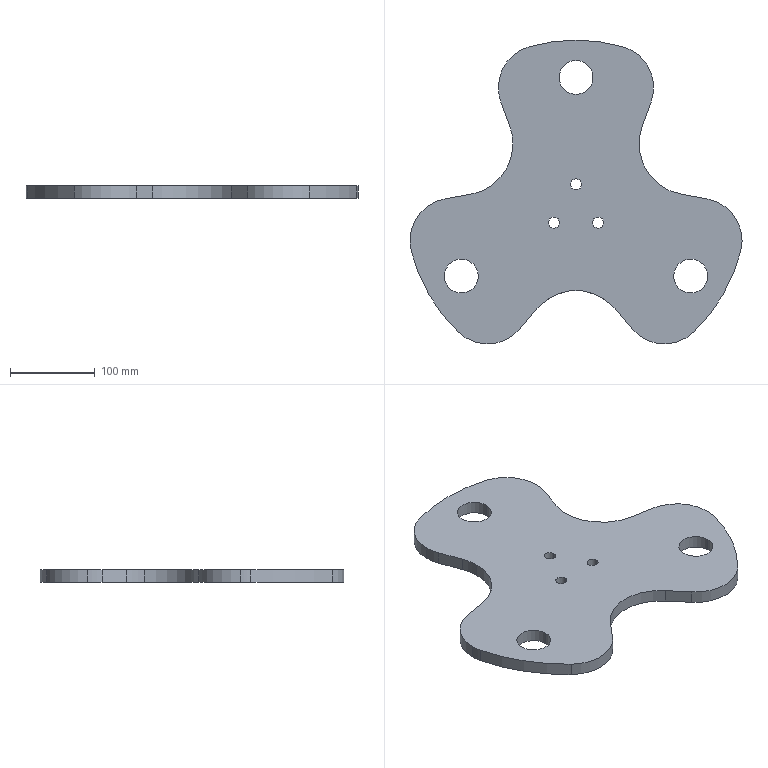Part | SolidWorks | features ICE 2, Extrusion 1, Fillet 1 | 1 solid | 35 faces | box 391.135 x 357.967 x 15 mm | volume 1196806 mm3 | cylinder 27 | plane 8 | commonest cylinder face diameters 100 x8 13 x6 40 x6 120 x4 400 x3
STEP:
#1=CARTESIAN_POINT('',(-6.5,30.,0.));
#2=VERTEX_POINT('',#1);
#3=CARTESIAN_POINT('',(6.5,30.,0.));
#4=VERTEX_POINT('',#3);
#5=CARTESIAN_POINT('',(0.,30.,0.));
#6=DIRECTION('',(0.,0.,1.));
#7=DIRECTION('',(1.,0.,0.));
#8=AXIS2_PLACEMENT_3D('',#5,#6,#7);
#9=CIRCLE('',#8,6.5);
#10=EDGE_CURVE('',#2,#4,#9,.T.);
#11=ORIENTED_EDGE('',*,*,#10,.F.);
#12=CARTESIAN_POINT('',(-6.5,30.,15.));
#13=VERTEX_POINT('',#12);
#14=CARTESIAN_POINT('',(-6.5,30.,-35.));
#15=DIRECTION('',(0.,0.,1.));
#16=VECTOR('',#15,1000.);
#17=LINE('',#14,#16);
#18=EDGE_CURVE('',#2,#13,#17,.T.);
#19=ORIENTED_EDGE('',*,*,#18,.T.);
#20=CARTESIAN_POINT('',(6.5,30.,15.));
#21=VERTEX_POINT('',#20);
#22=CARTESIAN_POINT('',(0.,30.,15.));
#23=DIRECTION('',(0.,0.,1.));
#24=DIRECTION('',(1.,0.,0.));
#25=AXIS2_PLACEMENT_3D('',#22,#23,#24);
#26=CIRCLE('',#25,6.5);
#27=EDGE_CURVE('',#13,#21,#26,.T.);
#28=ORIENTED_EDGE('',*,*,#27,.T.);
#29=CARTESIAN_POINT('',(6.5,30.,-35.));
#30=DIRECTION('',(0.,0.,1.));
#31=VECTOR('',#30,1000.);
#32=LINE('',#29,#31);
#33=EDGE_CURVE('',#4,#21,#32,.T.);
#34=ORIENTED_EDGE('',*,*,#33,.F.);
#35=EDGE_LOOP('',(#11,#19,#28,#34));
#36=FACE_OUTER_BOUND('',#35,.T.);
#37=CARTESIAN_POINT('',(0.,30.,-35.));
#38=DIRECTION('',(0.,0.,1.));
#39=DIRECTION('',(1.,0.,0.));
#40=AXIS2_PLACEMENT_3D('',#37,#38,#39);
#41=CYLINDRICAL_SURFACE('',#40,6.5);
#42=ADVANCED_FACE('',(#36),#41,.F.);
#43=CARTESIAN_POINT('',(19.481,-15.,0.));
#44=VERTEX_POINT('',#43);
#45=CARTESIAN_POINT('',(32.481,-15.,0.));
#46=VERTEX_POINT('',#45);
#47=CARTESIAN_POINT('',(25.981,-15.,0.));
#48=DIRECTION('',(0.,0.,1.));
#49=DIRECTION('',(1.,0.,0.));
#50=AXIS2_PLACEMENT_3D('',#47,#48,#49);
#51=CIRCLE('',#50,6.5);
#52=EDGE_CURVE('',#44,#46,#51,.T.);
#53=ORIENTED_EDGE('',*,*,#52,.F.);
#54=CARTESIAN_POINT('',(19.481,-15.,15.));
#55=VERTEX_POINT('',#54);
#56=CARTESIAN_POINT('',(19.481,-15.,-35.));
#57=DIRECTION('',(0.,0.,1.));
#58=VECTOR('',#57,1000.);
#59=LINE('',#56,#58);
#60=EDGE_CURVE('',#44,#55,#59,.T.);
#61=ORIENTED_EDGE('',*,*,#60,.T.);
#62=CARTESIAN_POINT('',(32.481,-15.,15.));
#63=VERTEX_POINT('',#62);
#64=CARTESIAN_POINT('',(25.981,-15.,15.));
#65=DIRECTION('',(0.,0.,1.));
#66=DIRECTION('',(1.,0.,0.));
#67=AXIS2_PLACEMENT_3D('',#64,#65,#66);
#68=CIRCLE('',#67,6.5);
#69=EDGE_CURVE('',#55,#63,#68,.T.);
#70=ORIENTED_EDGE('',*,*,#69,.T.);
#71=CARTESIAN_POINT('',(32.481,-15.,-35.));
#72=DIRECTION('',(0.,0.,1.));
#73=VECTOR('',#72,1000.);
#74=LINE('',#71,#73);
#75=EDGE_CURVE('',#46,#63,#74,.T.);
#76=ORIENTED_EDGE('',*,*,#75,.F.);
#77=EDGE_LOOP('',(#53,#61,#70,#76));
#78=FACE_OUTER_BOUND('',#77,.T.);
#79=CARTESIAN_POINT('',(25.981,-15.,-35.));
#80=DIRECTION('',(0.,0.,1.));
#81=DIRECTION('',(1.,0.,0.));
#82=AXIS2_PLACEMENT_3D('',#79,#80,#81);
#83=CYLINDRICAL_SURFACE('',#82,6.5);
#84=ADVANCED_FACE('',(#78),#83,.F.);
#85=CARTESIAN_POINT('',(-32.481,-15.,0.));
#86=VERTEX_POINT('',#85);
#87=CARTESIAN_POINT('',(-19.481,-15.,0.));
#88=VERTEX_POINT('',#87);
#89=CARTESIAN_POINT('',(-25.981,-15.,0.));
#90=DIRECTION('',(0.,0.,1.));
#91=DIRECTION('',(1.,0.,0.));
#92=AXIS2_PLACEMENT_3D('',#89,#90,#91);
#93=CIRCLE('',#92,6.5);
#94=EDGE_CURVE('',#86,#88,#93,.T.);
#95=ORIENTED_EDGE('',*,*,#94,.F.);
#96=CARTESIAN_POINT('',(-32.481,-15.,15.));
#97=VERTEX_POINT('',#96);
#98=CARTESIAN_POINT('',(-32.481,-15.,-35.));
#99=DIRECTION('',(0.,0.,1.));
#100=VECTOR('',#99,1000.);
#101=LINE('',#98,#100);
#102=EDGE_CURVE('',#86,#97,#101,.T.);
#103=ORIENTED_EDGE('',*,*,#102,.T.);
#104=CARTESIAN_POINT('',(-19.481,-15.,15.));
#105=VERTEX_POINT('',#104);
#106=CARTESIAN_POINT('',(-25.981,-15.,15.));
#107=DIRECTION('',(0.,0.,1.));
#108=DIRECTION('',(1.,0.,0.));
#109=AXIS2_PLACEMENT_3D('',#106,#107,#108);
#110=CIRCLE('',#109,6.5);
#111=EDGE_CURVE('',#97,#105,#110,.T.);
#112=ORIENTED_EDGE('',*,*,#111,.T.);
#113=CARTESIAN_POINT('',(-19.481,-15.,-35.));
#114=DIRECTION('',(0.,0.,1.));
#115=VECTOR('',#114,1000.);
#116=LINE('',#113,#115);
#117=EDGE_CURVE('',#88,#105,#116,.T.);
#118=ORIENTED_EDGE('',*,*,#117,.F.);
#119=EDGE_LOOP('',(#95,#103,#112,#118));
#120=FACE_OUTER_BOUND('',#119,.T.);
#121=CARTESIAN_POINT('',(-25.981,-15.,-35.));
#122=DIRECTION('',(0.,0.,1.));
#123=DIRECTION('',(1.,0.,0.));
#124=AXIS2_PLACEMENT_3D('',#121,#122,#123);
#125=CYLINDRICAL_SURFACE('',#124,6.5);
#126=ADVANCED_FACE('',(#120),#125,.F.);
#127=CARTESIAN_POINT('',(-91.438,144.163,15.));
#128=VERTEX_POINT('',#127);
#129=CARTESIAN_POINT('',(-88.422,127.062,15.));
#130=VERTEX_POINT('',#129);
#131=CARTESIAN_POINT('',(-41.438,144.163,15.));
#132=DIRECTION('',(0.,0.,1.));
#133=DIRECTION('',(1.,0.,0.));
#134=AXIS2_PLACEMENT_3D('',#131,#132,#133);
#135=CIRCLE('',#134,50.);
#136=EDGE_CURVE('',#128,#130,#135,.T.);
#137=ORIENTED_EDGE('',*,*,#136,.F.);
#138=CARTESIAN_POINT('',(-91.438,144.163,0.));
#139=VERTEX_POINT('',#138);
#140=CARTESIAN_POINT('',(-91.438,144.163,15.));
#141=DIRECTION('',(0.,0.,-1.));
#142=VECTOR('',#141,1000.);
#143=LINE('',#140,#142);
#144=EDGE_CURVE('',#128,#139,#143,.T.);
#145=ORIENTED_EDGE('',*,*,#144,.T.);
#146=CARTESIAN_POINT('',(-88.422,127.062,0.));
#147=VERTEX_POINT('',#146);
#148=CARTESIAN_POINT('',(-41.438,144.163,0.));
#149=DIRECTION('',(0.,0.,-1.));
#150=DIRECTION('',(1.,0.,0.));
#151=AXIS2_PLACEMENT_3D('',#148,#149,#150);
#152=CIRCLE('',#151,50.);
#153=EDGE_CURVE('',#147,#139,#152,.T.);
#154=ORIENTED_EDGE('',*,*,#153,.F.);
#155=CARTESIAN_POINT('',(-88.422,127.062,-15.));
#156=DIRECTION('',(0.,0.,-1.));
#157=VECTOR('',#156,1000.);
#158=LINE('',#155,#157);
#159=EDGE_CURVE('',#130,#147,#158,.T.);
#160=ORIENTED_EDGE('',*,*,#159,.F.);
#161=EDGE_LOOP('',(#137,#145,#154,#160));
#162=FACE_OUTER_BOUND('',#161,.T.);
#163=CARTESIAN_POINT('',(-41.438,144.163,15.));
#164=DIRECTION('',(0.,0.,-1.));
#165=DIRECTION('',(-1.,0.,0.));
#166=AXIS2_PLACEMENT_3D('',#163,#164,#165);
#167=CYLINDRICAL_SURFACE('',#166,50.);
#168=ADVANCED_FACE('',(#162),#167,.T.);
#169=CARTESIAN_POINT('',(-195.568,-36.195,15.));
#170=VERTEX_POINT('',#169);
#171=CARTESIAN_POINT('',(-194.09,-48.26,15.));
#172=VERTEX_POINT('',#171);
#173=CARTESIAN_POINT('',(-145.568,-36.195,15.));
#174=DIRECTION('',(0.,0.,1.));
#175=DIRECTION('',(1.,0.,0.));
#176=AXIS2_PLACEMENT_3D('',#173,#174,#175);
#177=CIRCLE('',#176,50.);
#178=EDGE_CURVE('',#170,#172,#177,.T.);
#179=ORIENTED_EDGE('',*,*,#178,.F.);
#180=CARTESIAN_POINT('',(-195.568,-36.195,0.));
#181=VERTEX_POINT('',#180);
#182=CARTESIAN_POINT('',(-195.568,-36.195,15.));
#183=DIRECTION('',(0.,0.,-1.));
#184=VECTOR('',#183,1000.);
#185=LINE('',#182,#184);
#186=EDGE_CURVE('',#170,#181,#185,.T.);
#187=ORIENTED_EDGE('',*,*,#186,.T.);
#188=CARTESIAN_POINT('',(-194.09,-48.26,0.));
#189=VERTEX_POINT('',#188);
#190=CARTESIAN_POINT('',(-145.568,-36.195,0.));
#191=DIRECTION('',(0.,0.,-1.));
#192=DIRECTION('',(1.,0.,0.));
#193=AXIS2_PLACEMENT_3D('',#190,#191,#192);
#194=CIRCLE('',#193,50.);
#195=EDGE_CURVE('',#189,#181,#194,.T.);
#196=ORIENTED_EDGE('',*,*,#195,.F.);
#197=CARTESIAN_POINT('',(-194.09,-48.26,15.));
#198=DIRECTION('',(0.,0.,-1.));
#199=VECTOR('',#198,1000.);
#200=LINE('',#197,#199);
#201=EDGE_CURVE('',#172,#189,#200,.T.);
#202=ORIENTED_EDGE('',*,*,#201,.F.);
#203=EDGE_LOOP('',(#179,#187,#196,#202));
#204=FACE_OUTER_BOUND('',#203,.T.);
#205=CARTESIAN_POINT('',(-145.568,-36.195,15.));
#206=DIRECTION('',(0.,0.,-1.));
#207=DIRECTION('',(-1.,0.,0.));
#208=AXIS2_PLACEMENT_3D('',#205,#206,#207);
#209=CYLINDRICAL_SURFACE('',#208,50.);
#210=ADVANCED_FACE('',(#204),#209,.T.);
#211=CARTESIAN_POINT('',(-74.234,77.5,0.));
#212=VERTEX_POINT('',#211);
#213=CARTESIAN_POINT('',(-77.852,98.021,0.));
#214=VERTEX_POINT('',#213);
#215=CARTESIAN_POINT('',(-134.234,77.5,0.));
#216=DIRECTION('',(0.,0.,1.));
#217=DIRECTION('',(1.,0.,0.));
#218=AXIS2_PLACEMENT_3D('',#215,#216,#217);
#219=CIRCLE('',#218,60.);
#220=EDGE_CURVE('',#212,#214,#219,.T.);
#221=ORIENTED_EDGE('',*,*,#220,.F.);
#222=CARTESIAN_POINT('',(-74.234,77.5,15.));
#223=VERTEX_POINT('',#222);
#224=CARTESIAN_POINT('',(-74.234,77.5,-15.));
#225=DIRECTION('',(0.,0.,1.));
#226=VECTOR('',#225,1000.);
#227=LINE('',#224,#226);
#228=EDGE_CURVE('',#212,#223,#227,.T.);
#229=ORIENTED_EDGE('',*,*,#228,.T.);
#230=CARTESIAN_POINT('',(-77.852,98.021,15.));
#231=VERTEX_POINT('',#230);
#232=CARTESIAN_POINT('',(-134.234,77.5,15.));
#233=DIRECTION('',(0.,0.,1.));
#234=DIRECTION('',(-1.,0.,0.));
#235=AXIS2_PLACEMENT_3D('',#232,#233,#234);
#236=CIRCLE('',#235,60.);
#237=EDGE_CURVE('',#223,#231,#236,.T.);
#238=ORIENTED_EDGE('',*,*,#237,.T.);
#239=CARTESIAN_POINT('',(-77.852,98.021,-15.));
#240=DIRECTION('',(0.,0.,1.));
#241=VECTOR('',#240,1000.);
#242=LINE('',#239,#241);
#243=EDGE_CURVE('',#214,#231,#242,.T.);
#244=ORIENTED_EDGE('',*,*,#243,.F.);
#245=EDGE_LOOP('',(#221,#229,#238,#244));
#246=FACE_OUTER_BOUND('',#245,.T.);
#247=CARTESIAN_POINT('',(-134.234,77.5,-15.));
#248=DIRECTION('',(0.,0.,1.));
#249=DIRECTION('',(1.,0.,0.));
#250=AXIS2_PLACEMENT_3D('',#247,#248,#249);
#251=CYLINDRICAL_SURFACE('',#250,60.);
#252=ADVANCED_FACE('',(#246),#251,.F.);
#253=CARTESIAN_POINT('',(-155.1,-78.,15.));
#254=VERTEX_POINT('',#253);
#255=CARTESIAN_POINT('',(-115.1,-78.,15.));
#256=VERTEX_POINT('',#255);
#257=CARTESIAN_POINT('',(-135.1,-78.,15.));
#258=DIRECTION('',(0.,0.,1.));
#259=DIRECTION('',(1.,0.,0.));
#260=AXIS2_PLACEMENT_3D('',#257,#258,#259);
#261=CIRCLE('',#260,20.);
#262=EDGE_CURVE('',#254,#256,#261,.T.);
#263=ORIENTED_EDGE('',*,*,#262,.T.);
#264=CARTESIAN_POINT('',(-115.1,-78.,0.));
#265=VERTEX_POINT('',#264);
#266=CARTESIAN_POINT('',(-115.1,-78.,15.));
#267=DIRECTION('',(0.,0.,-1.));
#268=VECTOR('',#267,1000.);
#269=LINE('',#266,#268);
#270=EDGE_CURVE('',#256,#265,#269,.T.);
#271=ORIENTED_EDGE('',*,*,#270,.T.);
#272=CARTESIAN_POINT('',(-155.1,-78.,0.));
#273=VERTEX_POINT('',#272);
#274=CARTESIAN_POINT('',(-135.1,-78.,0.));
#275=DIRECTION('',(0.,0.,1.));
#276=DIRECTION('',(1.,0.,0.));
#277=AXIS2_PLACEMENT_3D('',#274,#275,#276);
#278=CIRCLE('',#277,20.);
#279=EDGE_CURVE('',#273,#265,#278,.T.);
#280=ORIENTED_EDGE('',*,*,#279,.F.);
#281=CARTESIAN_POINT('',(-155.1,-78.,15.));
#282=DIRECTION('',(0.,0.,-1.));
#283=VECTOR('',#282,1000.);
#284=LINE('',#281,#283);
#285=EDGE_CURVE('',#254,#273,#284,.T.);
#286=ORIENTED_EDGE('',*,*,#285,.F.);
#287=EDGE_LOOP('',(#263,#271,#280,#286));
#288=FACE_OUTER_BOUND('',#287,.T.);
#289=CARTESIAN_POINT('',(-135.1,-78.,15.));
#290=DIRECTION('',(0.,0.,-1.));
#291=DIRECTION('',(-1.,0.,0.));
#292=AXIS2_PLACEMENT_3D('',#289,#290,#291);
#293=CYLINDRICAL_SURFACE('',#292,20.);
#294=ADVANCED_FACE('',(#288),#293,.F.);
#295=CARTESIAN_POINT('',(115.1,-78.,15.));
#296=VERTEX_POINT('',#295);
#297=CARTESIAN_POINT('',(155.1,-78.,15.));
#298=VERTEX_POINT('',#297);
#299=CARTESIAN_POINT('',(135.1,-78.,15.));
#300=DIRECTION('',(0.,0.,1.));
#301=DIRECTION('',(1.,0.,0.));
#302=AXIS2_PLACEMENT_3D('',#299,#300,#301);
#303=CIRCLE('',#302,20.);
#304=EDGE_CURVE('',#296,#298,#303,.T.);
#305=ORIENTED_EDGE('',*,*,#304,.T.);
#306=CARTESIAN_POINT('',(155.1,-78.,0.));
#307=VERTEX_POINT('',#306);
#308=CARTESIAN_POINT('',(155.1,-78.,15.));
#309=DIRECTION('',(0.,0.,-1.));
#310=VECTOR('',#309,1000.);
#311=LINE('',#308,#310);
#312=EDGE_CURVE('',#298,#307,#311,.T.);
#313=ORIENTED_EDGE('',*,*,#312,.T.);
#314=CARTESIAN_POINT('',(115.1,-78.,0.));
#315=VERTEX_POINT('',#314);
#316=CARTESIAN_POINT('',(135.1,-78.,0.));
#317=DIRECTION('',(0.,0.,1.));
#318=DIRECTION('',(1.,0.,0.));
#319=AXIS2_PLACEMENT_3D('',#316,#317,#318);
#320=CIRCLE('',#319,20.);
#321=EDGE_CURVE('',#315,#307,#320,.T.);
#322=ORIENTED_EDGE('',*,*,#321,.F.);
#323=CARTESIAN_POINT('',(115.1,-78.,15.));
#324=DIRECTION('',(0.,0.,-1.));
#325=VECTOR('',#324,1000.);
#326=LINE('',#323,#325);
#327=EDGE_CURVE('',#296,#315,#326,.T.);
#328=ORIENTED_EDGE('',*,*,#327,.F.);
#329=EDGE_LOOP('',(#305,#313,#322,#328));
#330=FACE_OUTER_BOUND('',#329,.T.);
#331=CARTESIAN_POINT('',(135.1,-78.,15.));
#332=DIRECTION('',(0.,0.,-1.));
#333=DIRECTION('',(-1.,0.,0.));
#334=AXIS2_PLACEMENT_3D('',#331,#332,#333);
#335=CYLINDRICAL_SURFACE('',#334,20.);
#336=ADVANCED_FACE('',(#330),#335,.F.);
#337=CARTESIAN_POINT('',(-20.,156.,15.));
#338=VERTEX_POINT('',#337);
#339=CARTESIAN_POINT('',(20.,156.,15.));
#340=VERTEX_POINT('',#339);
#341=CARTESIAN_POINT('',(0.,156.,15.));
#342=DIRECTION('',(0.,0.,1.));
#343=DIRECTION('',(1.,0.,0.));
#344=AXIS2_PLACEMENT_3D('',#341,#342,#343);
#345=CIRCLE('',#344,20.);
#346=EDGE_CURVE('',#338,#340,#345,.T.);
#347=ORIENTED_EDGE('',*,*,#346,.T.);
#348=CARTESIAN_POINT('',(20.,156.,0.));
#349=VERTEX_POINT('',#348);
#350=CARTESIAN_POINT('',(20.,156.,15.));
#351=DIRECTION('',(0.,0.,-1.));
#352=VECTOR('',#351,1000.);
#353=LINE('',#350,#352);
#354=EDGE_CURVE('',#340,#349,#353,.T.);
#355=ORIENTED_EDGE('',*,*,#354,.T.);
#356=CARTESIAN_POINT('',(-20.,156.,0.));
#357=VERTEX_POINT('',#356);
#358=CARTESIAN_POINT('',(0.,156.,0.));
#359=DIRECTION('',(0.,0.,1.));
#360=DIRECTION('',(1.,0.,0.));
#361=AXIS2_PLACEMENT_3D('',#358,#359,#360);
#362=CIRCLE('',#361,20.);
#363=EDGE_CURVE('',#357,#349,#362,.T.);
#364=ORIENTED_EDGE('',*,*,#363,.F.);
#365=CARTESIAN_POINT('',(-20.,156.,15.));
#366=DIRECTION('',(0.,0.,-1.));
#367=VECTOR('',#366,1000.);
#368=LINE('',#365,#367);
#369=EDGE_CURVE('',#338,#357,#368,.T.);
#370=ORIENTED_EDGE('',*,*,#369,.F.);
#371=EDGE_LOOP('',(#347,#355,#364,#370));
#372=FACE_OUTER_BOUND('',#371,.T.);
#373=CARTESIAN_POINT('',(0.,156.,15.));
#374=DIRECTION('',(0.,0.,-1.));
#375=DIRECTION('',(-1.,0.,0.));
#376=AXIS2_PLACEMENT_3D('',#373,#374,#375);
#377=CYLINDRICAL_SURFACE('',#376,20.);
#378=ADVANCED_FACE('',(#372),#377,.F.);
#379=CARTESIAN_POINT('',(138.84,-143.957,15.));
#380=VERTEX_POINT('',#379);
#381=CARTESIAN_POINT('',(194.09,-48.26,15.));
#382=VERTEX_POINT('',#381);
#383=CARTESIAN_POINT('',(0.,0.,15.));
#384=DIRECTION('',(0.,0.,1.));
#385=DIRECTION('',(1.,0.,0.));
#386=AXIS2_PLACEMENT_3D('',#383,#384,#385);
#387=CIRCLE('',#386,200.);
#388=EDGE_CURVE('',#380,#382,#387,.T.);
#389=ORIENTED_EDGE('',*,*,#388,.F.);
#390=CARTESIAN_POINT('',(138.84,-143.957,0.));
#391=VERTEX_POINT('',#390);
#392=CARTESIAN_POINT('',(138.84,-143.957,15.));
#393=DIRECTION('',(0.,0.,-1.));
#394=VECTOR('',#393,1000.);
#395=LINE('',#392,#394);
#396=EDGE_CURVE('',#380,#391,#395,.T.);
#397=ORIENTED_EDGE('',*,*,#396,.T.);
#398=CARTESIAN_POINT('',(194.09,-48.26,0.));
#399=VERTEX_POINT('',#398);
#400=CARTESIAN_POINT('',(0.,0.,0.));
#401=DIRECTION('',(0.,0.,1.));
#402=DIRECTION('',(1.,0.,0.));
#403=AXIS2_PLACEMENT_3D('',#400,#401,#402);
#404=CIRCLE('',#403,200.);
#405=EDGE_CURVE('',#391,#399,#404,.T.);
#406=ORIENTED_EDGE('',*,*,#405,.T.);
#407=CARTESIAN_POINT('',(194.09,-48.26,15.));
#408=DIRECTION('',(0.,0.,1.));
#409=VECTOR('',#408,1000.);
#410=LINE('',#407,#409);
#411=EDGE_CURVE('',#399,#382,#410,.T.);
#412=ORIENTED_EDGE('',*,*,#411,.T.);
#413=EDGE_LOOP('',(#389,#397,#406,#412));
#414=FACE_OUTER_BOUND('',#413,.T.);
#415=CARTESIAN_POINT('',(0.,0.,15.));
#416=DIRECTION('',(0.,0.,-1.));
#417=DIRECTION('',(-1.,0.,0.));
#418=AXIS2_PLACEMENT_3D('',#415,#416,#417);
#419=CYLINDRICAL_SURFACE('',#418,200.);
#420=ADVANCED_FACE('',(#414),#419,.T.);
#421=CARTESIAN_POINT('',(-138.84,-143.957,0.));
#422=VERTEX_POINT('',#421);
#423=CARTESIAN_POINT('',(0.,0.,0.));
#424=DIRECTION('',(0.,0.,1.));
#425=DIRECTION('',(1.,0.,0.));
#426=AXIS2_PLACEMENT_3D('',#423,#424,#425);
#427=CIRCLE('',#426,200.);
#428=EDGE_CURVE('',#189,#422,#427,.T.);
#429=ORIENTED_EDGE('',*,*,#428,.T.);
#430=CARTESIAN_POINT('',(-138.84,-143.957,15.));
#431=VERTEX_POINT('',#430);
#432=CARTESIAN_POINT('',(-138.84,-143.957,15.));
#433=DIRECTION('',(0.,0.,1.));
#434=VECTOR('',#433,1000.);
#435=LINE('',#432,#434);
#436=EDGE_CURVE('',#422,#431,#435,.T.);
#437=ORIENTED_EDGE('',*,*,#436,.T.);
#438=CARTESIAN_POINT('',(0.,0.,15.));
#439=DIRECTION('',(0.,0.,1.));
#440=DIRECTION('',(1.,0.,0.));
#441=AXIS2_PLACEMENT_3D('',#438,#439,#440);
#442=CIRCLE('',#441,200.);
#443=EDGE_CURVE('',#172,#431,#442,.T.);
#444=ORIENTED_EDGE('',*,*,#443,.F.);
#445=ORIENTED_EDGE('',*,*,#201,.T.);
#446=EDGE_LOOP('',(#429,#437,#444,#445));
#447=FACE_OUTER_BOUND('',#446,.T.);
#448=CARTESIAN_POINT('',(0.,0.,15.));
#449=DIRECTION('',(0.,0.,-1.));
#450=DIRECTION('',(-1.,0.,0.));
#451=AXIS2_PLACEMENT_3D('',#448,#449,#450);
#452=CYLINDRICAL_SURFACE('',#451,200.);
#453=ADVANCED_FACE('',(#447),#452,.T.);
#454=CARTESIAN_POINT('',(0.,30.,15.));
#455=DIRECTION('',(0.,0.,1.));
#456=DIRECTION('',(1.,0.,0.));
#457=AXIS2_PLACEMENT_3D('',#454,#455,#456);
#458=CIRCLE('',#457,6.5);
#459=EDGE_CURVE('',#21,#13,#458,.T.);
#460=ORIENTED_EDGE('',*,*,#459,.F.);
#461=ORIENTED_EDGE('',*,*,#27,.F.);
#462=EDGE_LOOP('',(#460,#461));
#463=FACE_BOUND('',#462,.T.);
#464=CARTESIAN_POINT('',(25.981,-15.,15.));
#465=DIRECTION('',(0.,0.,1.));
#466=DIRECTION('',(1.,0.,0.));
#467=AXIS2_PLACEMENT_3D('',#464,#465,#466);
#468=CIRCLE('',#467,6.5);
#469=EDGE_CURVE('',#63,#55,#468,.T.);
#470=ORIENTED_EDGE('',*,*,#469,.F.);
#471=ORIENTED_EDGE('',*,*,#69,.F.);
#472=EDGE_LOOP('',(#470,#471));
#473=FACE_BOUND('',#472,.T.);
#474=CARTESIAN_POINT('',(-25.981,-15.,15.));
#475=DIRECTION('',(0.,0.,1.));
#476=DIRECTION('',(1.,0.,0.));
#477=AXIS2_PLACEMENT_3D('',#474,#475,#476);
#478=CIRCLE('',#477,6.5);
#479=EDGE_CURVE('',#105,#97,#478,.T.);
#480=ORIENTED_EDGE('',*,*,#479,.F.);
#481=ORIENTED_EDGE('',*,*,#111,.F.);
#482=EDGE_LOOP('',(#480,#481));
#483=FACE_BOUND('',#482,.T.);
#484=ORIENTED_EDGE('',*,*,#443,.T.);
#485=CARTESIAN_POINT('',(-65.828,-140.107,15.));
#486=VERTEX_POINT('',#485);
#487=CARTESIAN_POINT('',(-104.13,-107.967,15.));
#488=DIRECTION('',(0.,0.,1.));
#489=DIRECTION('',(1.,0.,0.));
#490=AXIS2_PLACEMENT_3D('',#487,#488,#489);
#491=CIRCLE('',#490,50.);
#492=EDGE_CURVE('',#431,#486,#491,.T.);
#493=ORIENTED_EDGE('',*,*,#492,.T.);
#494=CARTESIAN_POINT('',(-45.963,-116.433,15.));
#495=VERTEX_POINT('',#494);
#496=CARTESIAN_POINT('',(-45.963,-116.433,15.));
#497=DIRECTION('',(-0.6428,-0.766,0.));
#498=VECTOR('',#497,1000.);
#499=LINE('',#496,#498);
#500=EDGE_CURVE('',#495,#486,#499,.T.);
#501=ORIENTED_EDGE('',*,*,#500,.F.);
#502=CARTESIAN_POINT('',(45.963,-116.433,15.));
#503=VERTEX_POINT('',#502);
#504=CARTESIAN_POINT('',(0.,-155.,15.));
#505=DIRECTION('',(0.,0.,1.));
#506=DIRECTION('',(-1.,0.,0.));
#507=AXIS2_PLACEMENT_3D('',#504,#505,#506);
#508=CIRCLE('',#507,60.);
#509=EDGE_CURVE('',#503,#495,#508,.T.);
#510=ORIENTED_EDGE('',*,*,#509,.F.);
#511=CARTESIAN_POINT('',(65.828,-140.107,15.));
#512=VERTEX_POINT('',#511);
#513=CARTESIAN_POINT('',(100.686,-181.649,15.));
#514=DIRECTION('',(-0.6428,0.766,0.));
#515=VECTOR('',#514,1000.);
#516=LINE('',#513,#515);
#517=EDGE_CURVE('',#512,#503,#516,.T.);
#518=ORIENTED_EDGE('',*,*,#517,.F.);
#519=CARTESIAN_POINT('',(104.13,-107.967,15.));
#520=DIRECTION('',(0.,0.,1.));
#521=DIRECTION('',(1.,0.,0.));
#522=AXIS2_PLACEMENT_3D('',#519,#520,#521);
#523=CIRCLE('',#522,50.);
#524=EDGE_CURVE('',#512,#380,#523,.T.);
#525=ORIENTED_EDGE('',*,*,#524,.T.);
#526=ORIENTED_EDGE('',*,*,#388,.T.);
#527=CARTESIAN_POINT('',(154.25,13.045,15.));
#528=VERTEX_POINT('',#527);
#529=CARTESIAN_POINT('',(145.568,-36.195,15.));
#530=DIRECTION('',(0.,0.,1.));
#531=DIRECTION('',(1.,0.,0.));
#532=AXIS2_PLACEMENT_3D('',#529,#530,#531);
#533=CIRCLE('',#532,50.);
#534=EDGE_CURVE('',#382,#528,#533,.T.);
#535=ORIENTED_EDGE('',*,*,#534,.T.);
#536=CARTESIAN_POINT('',(123.815,18.412,15.));
#537=VERTEX_POINT('',#536);
#538=CARTESIAN_POINT('',(123.815,18.412,15.));
#539=DIRECTION('',(0.9848,-0.1736,0.));
#540=VECTOR('',#539,1000.);
#541=LINE('',#538,#540);
#542=EDGE_CURVE('',#537,#528,#541,.T.);
#543=ORIENTED_EDGE('',*,*,#542,.F.);
#544=CARTESIAN_POINT('',(77.852,98.021,15.));
#545=VERTEX_POINT('',#544);
#546=CARTESIAN_POINT('',(134.234,77.5,15.));
#547=DIRECTION('',(0.,0.,1.));
#548=DIRECTION('',(-1.,0.,0.));
#549=AXIS2_PLACEMENT_3D('',#546,#547,#548);
#550=CIRCLE('',#549,60.);
#551=EDGE_CURVE('',#545,#537,#550,.T.);
#552=ORIENTED_EDGE('',*,*,#551,.F.);
#553=CARTESIAN_POINT('',(88.422,127.062,15.));
#554=VERTEX_POINT('',#553);
#555=CARTESIAN_POINT('',(106.97,178.021,15.));
#556=DIRECTION('',(-0.342,-0.9397,0.));
#557=VECTOR('',#556,1000.);
#558=LINE('',#555,#557);
#559=EDGE_CURVE('',#554,#545,#558,.T.);
#560=ORIENTED_EDGE('',*,*,#559,.F.);
#561=CARTESIAN_POINT('',(55.25,192.217,15.));
#562=VERTEX_POINT('',#561);
#563=CARTESIAN_POINT('',(41.438,144.163,15.));
#564=DIRECTION('',(0.,0.,1.));
#565=DIRECTION('',(1.,0.,0.));
#566=AXIS2_PLACEMENT_3D('',#563,#564,#565);
#567=CIRCLE('',#566,50.);
#568=EDGE_CURVE('',#554,#562,#567,.T.);
#569=ORIENTED_EDGE('',*,*,#568,.T.);
#570=CARTESIAN_POINT('',(-55.25,192.217,15.));
#571=VERTEX_POINT('',#570);
#572=CARTESIAN_POINT('',(0.,0.,15.));
#573=DIRECTION('',(0.,0.,1.));
#574=DIRECTION('',(1.,0.,0.));
#575=AXIS2_PLACEMENT_3D('',#572,#573,#574);
#576=CIRCLE('',#575,200.);
#577=EDGE_CURVE('',#562,#571,#576,.T.);
#578=ORIENTED_EDGE('',*,*,#577,.T.);
#579=CARTESIAN_POINT('',(-41.438,144.163,15.));
#580=DIRECTION('',(0.,0.,1.));
#581=DIRECTION('',(1.,0.,0.));
#582=AXIS2_PLACEMENT_3D('',#579,#580,#581);
#583=CIRCLE('',#582,50.);
#584=EDGE_CURVE('',#571,#128,#583,.T.);
#585=ORIENTED_EDGE('',*,*,#584,.T.);
#586=ORIENTED_EDGE('',*,*,#136,.T.);
#587=CARTESIAN_POINT('',(-77.852,98.021,15.));
#588=DIRECTION('',(-0.342,0.9397,0.));
#589=VECTOR('',#588,1000.);
#590=LINE('',#587,#589);
#591=EDGE_CURVE('',#231,#130,#590,.T.);
#592=ORIENTED_EDGE('',*,*,#591,.F.);
#593=ORIENTED_EDGE('',*,*,#237,.F.);
#594=CARTESIAN_POINT('',(-123.815,18.412,15.));
#595=VERTEX_POINT('',#594);
#596=CARTESIAN_POINT('',(-134.234,77.5,15.));
#597=DIRECTION('',(0.,0.,1.));
#598=DIRECTION('',(-1.,0.,0.));
#599=AXIS2_PLACEMENT_3D('',#596,#597,#598);
#600=CIRCLE('',#599,60.);
#601=EDGE_CURVE('',#595,#223,#600,.T.);
#602=ORIENTED_EDGE('',*,*,#601,.F.);
#603=CARTESIAN_POINT('',(-154.25,13.045,15.));
#604=VERTEX_POINT('',#603);
#605=CARTESIAN_POINT('',(-207.656,3.628,15.));
#606=DIRECTION('',(0.9848,0.1736,0.));
#607=VECTOR('',#606,1000.);
#608=LINE('',#605,#607);
#609=EDGE_CURVE('',#604,#595,#608,.T.);
#610=ORIENTED_EDGE('',*,*,#609,.F.);
#611=CARTESIAN_POINT('',(-145.568,-36.195,15.));
#612=DIRECTION('',(0.,0.,1.));
#613=DIRECTION('',(1.,0.,0.));
#614=AXIS2_PLACEMENT_3D('',#611,#612,#613);
#615=CIRCLE('',#614,50.);
#616=EDGE_CURVE('',#604,#170,#615,.T.);
#617=ORIENTED_EDGE('',*,*,#616,.T.);
#618=ORIENTED_EDGE('',*,*,#178,.T.);
#619=EDGE_LOOP('',(#484,#493,#501,#510,#518,#525,#526,#535,#543,#552,#560,#569,#578,#585,#586,#592,#593,#602,#610,#617,#618));
#620=FACE_OUTER_BOUND('',#619,.T.);
#621=ORIENTED_EDGE('',*,*,#304,.F.);
#622=CARTESIAN_POINT('',(135.1,-78.,15.));
#623=DIRECTION('',(0.,0.,1.));
#624=DIRECTION('',(1.,0.,0.));
#625=AXIS2_PLACEMENT_3D('',#622,#623,#624);
#626=CIRCLE('',#625,20.);
#627=EDGE_CURVE('',#298,#296,#626,.T.);
#628=ORIENTED_EDGE('',*,*,#627,.F.);
#629=EDGE_LOOP('',(#621,#628));
#630=FACE_BOUND('',#629,.T.);
#631=ORIENTED_EDGE('',*,*,#346,.F.);
#632=CARTESIAN_POINT('',(0.,156.,15.));
#633=DIRECTION('',(0.,0.,1.));
#634=DIRECTION('',(1.,0.,0.));
#635=AXIS2_PLACEMENT_3D('',#632,#633,#634);
#636=CIRCLE('',#635,20.);
#637=EDGE_CURVE('',#340,#338,#636,.T.);
#638=ORIENTED_EDGE('',*,*,#637,.F.);
#639=EDGE_LOOP('',(#631,#638));
#640=FACE_BOUND('',#639,.T.);
#641=ORIENTED_EDGE('',*,*,#262,.F.);
#642=CARTESIAN_POINT('',(-135.1,-78.,15.));
#643=DIRECTION('',(0.,0.,1.));
#644=DIRECTION('',(1.,0.,0.));
#645=AXIS2_PLACEMENT_3D('',#642,#643,#644);
#646=CIRCLE('',#645,20.);
#647=EDGE_CURVE('',#256,#254,#646,.T.);
#648=ORIENTED_EDGE('',*,*,#647,.F.);
#649=EDGE_LOOP('',(#641,#648));
#650=FACE_BOUND('',#649,.T.);
#651=CARTESIAN_POINT('',(0.,0.,15.));
#652=DIRECTION('',(0.,0.,1.));
#653=DIRECTION('',(1.,0.,0.));
#654=AXIS2_PLACEMENT_3D('',#651,#652,#653);
#655=PLANE('',#654);
#656=ADVANCED_FACE('',(#463,#473,#483,#620,#630,#640,#650),#655,.T.);
#657=CARTESIAN_POINT('',(0.,30.,0.));
#658=DIRECTION('',(0.,0.,1.));
#659=DIRECTION('',(1.,0.,0.));
#660=AXIS2_PLACEMENT_3D('',#657,#658,#659);
#661=CIRCLE('',#660,6.5);
#662=EDGE_CURVE('',#4,#2,#661,.T.);
#663=ORIENTED_EDGE('',*,*,#662,.T.);
#664=ORIENTED_EDGE('',*,*,#10,.T.);
#665=EDGE_LOOP('',(#663,#664));
#666=FACE_BOUND('',#665,.T.);
#667=CARTESIAN_POINT('',(25.981,-15.,0.));
#668=DIRECTION('',(0.,0.,1.));
#669=DIRECTION('',(1.,0.,0.));
#670=AXIS2_PLACEMENT_3D('',#667,#668,#669);
#671=CIRCLE('',#670,6.5);
#672=EDGE_CURVE('',#46,#44,#671,.T.);
#673=ORIENTED_EDGE('',*,*,#672,.T.);
#674=ORIENTED_EDGE('',*,*,#52,.T.);
#675=EDGE_LOOP('',(#673,#674));
#676=FACE_BOUND('',#675,.T.);
#677=CARTESIAN_POINT('',(-25.981,-15.,0.));
#678=DIRECTION('',(0.,0.,1.));
#679=DIRECTION('',(1.,0.,0.));
#680=AXIS2_PLACEMENT_3D('',#677,#678,#679);
#681=CIRCLE('',#680,6.5);
#682=EDGE_CURVE('',#88,#86,#681,.T.);
#683=ORIENTED_EDGE('',*,*,#682,.T.);
#684=ORIENTED_EDGE('',*,*,#94,.T.);
#685=EDGE_LOOP('',(#683,#684));
#686=FACE_BOUND('',#685,.T.);
#687=CARTESIAN_POINT('',(-45.963,-116.433,0.));
#688=VERTEX_POINT('',#687);
#689=CARTESIAN_POINT('',(-65.828,-140.107,0.));
#690=VERTEX_POINT('',#689);
#691=CARTESIAN_POINT('',(30.36,-25.475,0.));
#692=DIRECTION('',(-0.6428,-0.766,0.));
#693=VECTOR('',#692,1000.);
#694=LINE('',#691,#693);
#695=EDGE_CURVE('',#688,#690,#694,.T.);
#696=ORIENTED_EDGE('',*,*,#695,.T.);
#697=CARTESIAN_POINT('',(-104.13,-107.967,0.));
#698=DIRECTION('',(0.,0.,-1.));
#699=DIRECTION('',(1.,0.,0.));
#700=AXIS2_PLACEMENT_3D('',#697,#698,#699);
#701=CIRCLE('',#700,50.);
#702=EDGE_CURVE('',#690,#422,#701,.T.);
#703=ORIENTED_EDGE('',*,*,#702,.T.);
#704=ORIENTED_EDGE('',*,*,#428,.F.);
#705=ORIENTED_EDGE('',*,*,#195,.T.);
#706=CARTESIAN_POINT('',(-154.25,13.045,0.));
#707=VERTEX_POINT('',#706);
#708=CARTESIAN_POINT('',(-145.568,-36.195,0.));
#709=DIRECTION('',(0.,0.,-1.));
#710=DIRECTION('',(1.,0.,0.));
#711=AXIS2_PLACEMENT_3D('',#708,#709,#710);
#712=CIRCLE('',#711,50.);
#713=EDGE_CURVE('',#181,#707,#712,.T.);
#714=ORIENTED_EDGE('',*,*,#713,.T.);
#715=CARTESIAN_POINT('',(-123.815,18.412,0.));
#716=VERTEX_POINT('',#715);
#717=CARTESIAN_POINT('',(-6.882,39.03,0.));
#718=DIRECTION('',(0.9848,0.1736,0.));
#719=VECTOR('',#718,1000.);
#720=LINE('',#717,#719);
#721=EDGE_CURVE('',#707,#716,#720,.T.);
#722=ORIENTED_EDGE('',*,*,#721,.T.);
#723=CARTESIAN_POINT('',(-134.234,77.5,0.));
#724=DIRECTION('',(0.,0.,1.));
#725=DIRECTION('',(1.,0.,0.));
#726=AXIS2_PLACEMENT_3D('',#723,#724,#725);
#727=CIRCLE('',#726,60.);
#728=EDGE_CURVE('',#716,#212,#727,.T.);
#729=ORIENTED_EDGE('',*,*,#728,.T.);
#730=ORIENTED_EDGE('',*,*,#220,.T.);
#731=CARTESIAN_POINT('',(-37.242,-13.555,0.));
#732=DIRECTION('',(-0.342,0.9397,0.));
#733=VECTOR('',#732,1000.);
#734=LINE('',#731,#733);
#735=EDGE_CURVE('',#214,#147,#734,.T.);
#736=ORIENTED_EDGE('',*,*,#735,.T.);
#737=ORIENTED_EDGE('',*,*,#153,.T.);
#738=CARTESIAN_POINT('',(-55.25,192.217,0.));
#739=VERTEX_POINT('',#738);
#740=CARTESIAN_POINT('',(-41.438,144.163,0.));
#741=DIRECTION('',(0.,0.,-1.));
#742=DIRECTION('',(1.,0.,0.));
#743=AXIS2_PLACEMENT_3D('',#740,#741,#742);
#744=CIRCLE('',#743,50.);
#745=EDGE_CURVE('',#139,#739,#744,.T.);
#746=ORIENTED_EDGE('',*,*,#745,.T.);
#747=CARTESIAN_POINT('',(55.25,192.217,0.));
#748=VERTEX_POINT('',#747);
#749=CARTESIAN_POINT('',(0.,0.,0.));
#750=DIRECTION('',(0.,0.,1.));
#751=DIRECTION('',(1.,0.,0.));
#752=AXIS2_PLACEMENT_3D('',#749,#750,#751);
#753=CIRCLE('',#752,200.);
#754=EDGE_CURVE('',#748,#739,#753,.T.);
#755=ORIENTED_EDGE('',*,*,#754,.F.);
#756=CARTESIAN_POINT('',(88.422,127.062,0.));
#757=VERTEX_POINT('',#756);
#758=CARTESIAN_POINT('',(41.438,144.163,0.));
#759=DIRECTION('',(0.,0.,-1.));
#760=DIRECTION('',(1.,0.,0.));
#761=AXIS2_PLACEMENT_3D('',#758,#759,#760);
#762=CIRCLE('',#761,50.);
#763=EDGE_CURVE('',#748,#757,#762,.T.);
#764=ORIENTED_EDGE('',*,*,#763,.T.);
#765=CARTESIAN_POINT('',(77.852,98.021,0.));
#766=VERTEX_POINT('',#765);
#767=CARTESIAN_POINT('',(37.242,-13.555,0.));
#768=DIRECTION('',(-0.342,-0.9397,0.));
#769=VECTOR('',#768,1000.);
#770=LINE('',#767,#769);
#771=EDGE_CURVE('',#757,#766,#770,.T.);
#772=ORIENTED_EDGE('',*,*,#771,.T.);
#773=CARTESIAN_POINT('',(123.815,18.412,0.));
#774=VERTEX_POINT('',#773);
#775=CARTESIAN_POINT('',(134.234,77.5,0.));
#776=DIRECTION('',(0.,0.,1.));
#777=DIRECTION('',(1.,0.,0.));
#778=AXIS2_PLACEMENT_3D('',#775,#776,#777);
#779=CIRCLE('',#778,60.);
#780=EDGE_CURVE('',#766,#774,#779,.T.);
#781=ORIENTED_EDGE('',*,*,#780,.T.);
#782=CARTESIAN_POINT('',(154.25,13.045,0.));
#783=VERTEX_POINT('',#782);
#784=CARTESIAN_POINT('',(6.882,39.03,0.));
#785=DIRECTION('',(0.9848,-0.1736,0.));
#786=VECTOR('',#785,1000.);
#787=LINE('',#784,#786);
#788=EDGE_CURVE('',#774,#783,#787,.T.);
#789=ORIENTED_EDGE('',*,*,#788,.T.);
#790=CARTESIAN_POINT('',(145.568,-36.195,0.));
#791=DIRECTION('',(0.,0.,-1.));
#792=DIRECTION('',(1.,0.,0.));
#793=AXIS2_PLACEMENT_3D('',#790,#791,#792);
#794=CIRCLE('',#793,50.);
#795=EDGE_CURVE('',#783,#399,#794,.T.);
#796=ORIENTED_EDGE('',*,*,#795,.T.);
#797=ORIENTED_EDGE('',*,*,#405,.F.);
#798=CARTESIAN_POINT('',(65.828,-140.107,0.));
#799=VERTEX_POINT('',#798);
#800=CARTESIAN_POINT('',(104.13,-107.967,0.));
#801=DIRECTION('',(0.,0.,-1.));
#802=DIRECTION('',(1.,0.,0.));
#803=AXIS2_PLACEMENT_3D('',#800,#801,#802);
#804=CIRCLE('',#803,50.);
#805=EDGE_CURVE('',#391,#799,#804,.T.);
#806=ORIENTED_EDGE('',*,*,#805,.T.);
#807=CARTESIAN_POINT('',(45.963,-116.433,0.));
#808=VERTEX_POINT('',#807);
#809=CARTESIAN_POINT('',(-30.36,-25.475,0.));
#810=DIRECTION('',(-0.6428,0.766,0.));
#811=VECTOR('',#810,1000.);
#812=LINE('',#809,#811);
#813=EDGE_CURVE('',#799,#808,#812,.T.);
#814=ORIENTED_EDGE('',*,*,#813,.T.);
#815=CARTESIAN_POINT('',(0.,-155.,0.));
#816=DIRECTION('',(0.,0.,1.));
#817=DIRECTION('',(1.,0.,0.));
#818=AXIS2_PLACEMENT_3D('',#815,#816,#817);
#819=CIRCLE('',#818,60.);
#820=EDGE_CURVE('',#808,#688,#819,.T.);
#821=ORIENTED_EDGE('',*,*,#820,.T.);
#822=EDGE_LOOP('',(#696,#703,#704,#705,#714,#722,#729,#730,#736,#737,#746,#755,#764,#772,#781,#789,#796,#797,#806,#814,#821));
#823=FACE_OUTER_BOUND('',#822,.T.);
#824=ORIENTED_EDGE('',*,*,#363,.T.);
#825=CARTESIAN_POINT('',(0.,156.,0.));
#826=DIRECTION('',(0.,0.,1.));
#827=DIRECTION('',(1.,0.,0.));
#828=AXIS2_PLACEMENT_3D('',#825,#826,#827);
#829=CIRCLE('',#828,20.);
#830=EDGE_CURVE('',#349,#357,#829,.T.);
#831=ORIENTED_EDGE('',*,*,#830,.T.);
#832=EDGE_LOOP('',(#824,#831));
#833=FACE_BOUND('',#832,.T.);
#834=ORIENTED_EDGE('',*,*,#321,.T.);
#835=CARTESIAN_POINT('',(135.1,-78.,0.));
#836=DIRECTION('',(0.,0.,1.));
#837=DIRECTION('',(1.,0.,0.));
#838=AXIS2_PLACEMENT_3D('',#835,#836,#837);
#839=CIRCLE('',#838,20.);
#840=EDGE_CURVE('',#307,#315,#839,.T.);
#841=ORIENTED_EDGE('',*,*,#840,.T.);
#842=EDGE_LOOP('',(#834,#841));
#843=FACE_BOUND('',#842,.T.);
#844=ORIENTED_EDGE('',*,*,#279,.T.);
#845=CARTESIAN_POINT('',(-135.1,-78.,0.));
#846=DIRECTION('',(0.,0.,1.));
#847=DIRECTION('',(1.,0.,0.));
#848=AXIS2_PLACEMENT_3D('',#845,#846,#847);
#849=CIRCLE('',#848,20.);
#850=EDGE_CURVE('',#265,#273,#849,.T.);
#851=ORIENTED_EDGE('',*,*,#850,.T.);
#852=EDGE_LOOP('',(#844,#851));
#853=FACE_BOUND('',#852,.T.);
#854=CARTESIAN_POINT('',(0.,0.,0.));
#855=DIRECTION('',(0.,0.,1.));
#856=DIRECTION('',(1.,0.,0.));
#857=AXIS2_PLACEMENT_3D('',#854,#855,#856);
#858=PLANE('',#857);
#859=ADVANCED_FACE('',(#666,#676,#686,#823,#833,#843,#853),#858,.F.);
#860=ORIENTED_EDGE('',*,*,#577,.F.);
#861=CARTESIAN_POINT('',(55.25,192.217,15.));
#862=DIRECTION('',(0.,0.,-1.));
#863=VECTOR('',#862,1000.);
#864=LINE('',#861,#863);
#865=EDGE_CURVE('',#562,#748,#864,.T.);
#866=ORIENTED_EDGE('',*,*,#865,.T.);
#867=ORIENTED_EDGE('',*,*,#754,.T.);
#868=CARTESIAN_POINT('',(-55.25,192.217,15.));
#869=DIRECTION('',(0.,0.,1.));
#870=VECTOR('',#869,1000.);
#871=LINE('',#868,#870);
#872=EDGE_CURVE('',#739,#571,#871,.T.);
#873=ORIENTED_EDGE('',*,*,#872,.T.);
#874=EDGE_LOOP('',(#860,#866,#867,#873));
#875=FACE_OUTER_BOUND('',#874,.T.);
#876=CARTESIAN_POINT('',(0.,0.,15.));
#877=DIRECTION('',(0.,0.,-1.));
#878=DIRECTION('',(-1.,0.,0.));
#879=AXIS2_PLACEMENT_3D('',#876,#877,#878);
#880=CYLINDRICAL_SURFACE('',#879,200.);
#881=ADVANCED_FACE('',(#875),#880,.T.);
#882=ORIENTED_EDGE('',*,*,#354,.F.);
#883=ORIENTED_EDGE('',*,*,#637,.T.);
#884=ORIENTED_EDGE('',*,*,#369,.T.);
#885=ORIENTED_EDGE('',*,*,#830,.F.);
#886=EDGE_LOOP('',(#882,#883,#884,#885));
#887=FACE_OUTER_BOUND('',#886,.T.);
#888=CARTESIAN_POINT('',(0.,156.,15.));
#889=DIRECTION('',(0.,0.,-1.));
#890=DIRECTION('',(-1.,0.,0.));
#891=AXIS2_PLACEMENT_3D('',#888,#889,#890);
#892=CYLINDRICAL_SURFACE('',#891,20.);
#893=ADVANCED_FACE('',(#887),#892,.F.);
#894=ORIENTED_EDGE('',*,*,#312,.F.);
#895=ORIENTED_EDGE('',*,*,#627,.T.);
#896=ORIENTED_EDGE('',*,*,#327,.T.);
#897=ORIENTED_EDGE('',*,*,#840,.F.);
#898=EDGE_LOOP('',(#894,#895,#896,#897));
#899=FACE_OUTER_BOUND('',#898,.T.);
#900=CARTESIAN_POINT('',(135.1,-78.,15.));
#901=DIRECTION('',(0.,0.,-1.));
#902=DIRECTION('',(-1.,0.,0.));
#903=AXIS2_PLACEMENT_3D('',#900,#901,#902);
#904=CYLINDRICAL_SURFACE('',#903,20.);
#905=ADVANCED_FACE('',(#899),#904,.F.);
#906=ORIENTED_EDGE('',*,*,#270,.F.);
#907=ORIENTED_EDGE('',*,*,#647,.T.);
#908=ORIENTED_EDGE('',*,*,#285,.T.);
#909=ORIENTED_EDGE('',*,*,#850,.F.);
#910=EDGE_LOOP('',(#906,#907,#908,#909));
#911=FACE_OUTER_BOUND('',#910,.T.);
#912=CARTESIAN_POINT('',(-135.1,-78.,15.));
#913=DIRECTION('',(0.,0.,-1.));
#914=DIRECTION('',(-1.,0.,0.));
#915=AXIS2_PLACEMENT_3D('',#912,#913,#914);
#916=CYLINDRICAL_SURFACE('',#915,20.);
#917=ADVANCED_FACE('',(#911),#916,.F.);
#918=CARTESIAN_POINT('',(77.852,98.021,-15.));
#919=DIRECTION('',(0.,0.,1.));
#920=VECTOR('',#919,1000.);
#921=LINE('',#918,#920);
#922=EDGE_CURVE('',#766,#545,#921,.T.);
#923=ORIENTED_EDGE('',*,*,#922,.T.);
#924=ORIENTED_EDGE('',*,*,#551,.T.);
#925=CARTESIAN_POINT('',(123.815,18.412,-15.));
#926=DIRECTION('',(0.,0.,1.));
#927=VECTOR('',#926,1000.);
#928=LINE('',#925,#927);
#929=EDGE_CURVE('',#774,#537,#928,.T.);
#930=ORIENTED_EDGE('',*,*,#929,.F.);
#931=ORIENTED_EDGE('',*,*,#780,.F.);
#932=EDGE_LOOP('',(#923,#924,#930,#931));
#933=FACE_OUTER_BOUND('',#932,.T.);
#934=CARTESIAN_POINT('',(134.234,77.5,-15.));
#935=DIRECTION('',(0.,0.,1.));
#936=DIRECTION('',(1.,0.,0.));
#937=AXIS2_PLACEMENT_3D('',#934,#935,#936);
#938=CYLINDRICAL_SURFACE('',#937,60.);
#939=ADVANCED_FACE('',(#933),#938,.F.);
#940=ORIENTED_EDGE('',*,*,#771,.F.);
#941=CARTESIAN_POINT('',(88.422,127.062,-15.));
#942=DIRECTION('',(0.,0.,1.));
#943=VECTOR('',#942,1000.);
#944=LINE('',#941,#943);
#945=EDGE_CURVE('',#757,#554,#944,.T.);
#946=ORIENTED_EDGE('',*,*,#945,.T.);
#947=ORIENTED_EDGE('',*,*,#559,.T.);
#948=ORIENTED_EDGE('',*,*,#922,.F.);
#949=EDGE_LOOP('',(#940,#946,#947,#948));
#950=FACE_OUTER_BOUND('',#949,.T.);
#951=CARTESIAN_POINT('',(106.97,178.021,-15.));
#952=DIRECTION('',(-0.9397,0.342,0.));
#953=DIRECTION('',(-0.342,-0.9397,0.));
#954=AXIS2_PLACEMENT_3D('',#951,#952,#953);
#955=PLANE('',#954);
#956=ADVANCED_FACE('',(#950),#955,.F.);
#957=ORIENTED_EDGE('',*,*,#542,.T.);
#958=CARTESIAN_POINT('',(154.25,13.045,-15.));
#959=DIRECTION('',(0.,0.,-1.));
#960=VECTOR('',#959,1000.);
#961=LINE('',#958,#960);
#962=EDGE_CURVE('',#528,#783,#961,.T.);
#963=ORIENTED_EDGE('',*,*,#962,.T.);
#964=ORIENTED_EDGE('',*,*,#788,.F.);
#965=ORIENTED_EDGE('',*,*,#929,.T.);
#966=EDGE_LOOP('',(#957,#963,#964,#965));
#967=FACE_OUTER_BOUND('',#966,.T.);
#968=CARTESIAN_POINT('',(123.815,18.412,-15.));
#969=DIRECTION('',(-0.1736,-0.9848,0.));
#970=DIRECTION('',(0.9848,-0.1736,0.));
#971=AXIS2_PLACEMENT_3D('',#968,#969,#970);
#972=PLANE('',#971);
#973=ADVANCED_FACE('',(#967),#972,.F.);
#974=ORIENTED_EDGE('',*,*,#228,.F.);
#975=ORIENTED_EDGE('',*,*,#728,.F.);
#976=CARTESIAN_POINT('',(-123.815,18.412,-15.));
#977=DIRECTION('',(0.,0.,1.));
#978=VECTOR('',#977,1000.);
#979=LINE('',#976,#978);
#980=EDGE_CURVE('',#716,#595,#979,.T.);
#981=ORIENTED_EDGE('',*,*,#980,.T.);
#982=ORIENTED_EDGE('',*,*,#601,.T.);
#983=EDGE_LOOP('',(#974,#975,#981,#982));
#984=FACE_OUTER_BOUND('',#983,.T.);
#985=CARTESIAN_POINT('',(-134.234,77.5,-15.));
#986=DIRECTION('',(0.,0.,1.));
#987=DIRECTION('',(1.,0.,0.));
#988=AXIS2_PLACEMENT_3D('',#985,#986,#987);
#989=CYLINDRICAL_SURFACE('',#988,60.);
#990=ADVANCED_FACE('',(#984),#989,.F.);
#991=ORIENTED_EDGE('',*,*,#721,.F.);
#992=CARTESIAN_POINT('',(-154.25,13.045,-15.));
#993=DIRECTION('',(0.,0.,1.));
#994=VECTOR('',#993,1000.);
#995=LINE('',#992,#994);
#996=EDGE_CURVE('',#707,#604,#995,.T.);
#997=ORIENTED_EDGE('',*,*,#996,.T.);
#998=ORIENTED_EDGE('',*,*,#609,.T.);
#999=ORIENTED_EDGE('',*,*,#980,.F.);
#1000=EDGE_LOOP('',(#991,#997,#998,#999));
#1001=FACE_OUTER_BOUND('',#1000,.T.);
#1002=CARTESIAN_POINT('',(-207.656,3.628,-15.));
#1003=DIRECTION('',(0.1736,-0.9848,0.));
#1004=DIRECTION('',(0.9848,0.1736,0.));
#1005=AXIS2_PLACEMENT_3D('',#1002,#1003,#1004);
#1006=PLANE('',#1005);
#1007=ADVANCED_FACE('',(#1001),#1006,.F.);
#1008=ORIENTED_EDGE('',*,*,#591,.T.);
#1009=ORIENTED_EDGE('',*,*,#159,.T.);
#1010=ORIENTED_EDGE('',*,*,#735,.F.);
#1011=ORIENTED_EDGE('',*,*,#243,.T.);
#1012=EDGE_LOOP('',(#1008,#1009,#1010,#1011));
#1013=FACE_OUTER_BOUND('',#1012,.T.);
#1014=CARTESIAN_POINT('',(-77.852,98.021,-15.));
#1015=DIRECTION('',(0.9397,0.342,0.));
#1016=DIRECTION('',(-0.342,0.9397,0.));
#1017=AXIS2_PLACEMENT_3D('',#1014,#1015,#1016);
#1018=PLANE('',#1017);
#1019=ADVANCED_FACE('',(#1013),#1018,.F.);
#1020=CARTESIAN_POINT('',(45.963,-116.433,-15.));
#1021=DIRECTION('',(0.,0.,1.));
#1022=VECTOR('',#1021,1000.);
#1023=LINE('',#1020,#1022);
#1024=EDGE_CURVE('',#808,#503,#1023,.T.);
#1025=ORIENTED_EDGE('',*,*,#1024,.T.);
#1026=ORIENTED_EDGE('',*,*,#509,.T.);
#1027=CARTESIAN_POINT('',(-45.963,-116.433,-15.));
#1028=DIRECTION('',(0.,0.,1.));
#1029=VECTOR('',#1028,1000.);
#1030=LINE('',#1027,#1029);
#1031=EDGE_CURVE('',#688,#495,#1030,.T.);
#1032=ORIENTED_EDGE('',*,*,#1031,.F.);
#1033=ORIENTED_EDGE('',*,*,#820,.F.);
#1034=EDGE_LOOP('',(#1025,#1026,#1032,#1033));
#1035=FACE_OUTER_BOUND('',#1034,.T.);
#1036=CARTESIAN_POINT('',(0.,-155.,-15.));
#1037=DIRECTION('',(0.,0.,1.));
#1038=DIRECTION('',(1.,0.,0.));
#1039=AXIS2_PLACEMENT_3D('',#1036,#1037,#1038);
#1040=CYLINDRICAL_SURFACE('',#1039,60.);
#1041=ADVANCED_FACE('',(#1035),#1040,.F.);
#1042=ORIENTED_EDGE('',*,*,#813,.F.);
#1043=CARTESIAN_POINT('',(65.828,-140.107,-15.));
#1044=DIRECTION('',(0.,0.,1.));
#1045=VECTOR('',#1044,1000.);
#1046=LINE('',#1043,#1045);
#1047=EDGE_CURVE('',#799,#512,#1046,.T.);
#1048=ORIENTED_EDGE('',*,*,#1047,.T.);
#1049=ORIENTED_EDGE('',*,*,#517,.T.);
#1050=ORIENTED_EDGE('',*,*,#1024,.F.);
#1051=EDGE_LOOP('',(#1042,#1048,#1049,#1050));
#1052=FACE_OUTER_BOUND('',#1051,.T.);
#1053=CARTESIAN_POINT('',(100.686,-181.649,-15.));
#1054=DIRECTION('',(0.766,0.6428,0.));
#1055=DIRECTION('',(-0.6428,0.766,0.));
#1056=AXIS2_PLACEMENT_3D('',#1053,#1054,#1055);
#1057=PLANE('',#1056);
#1058=ADVANCED_FACE('',(#1052),#1057,.F.);
#1059=ORIENTED_EDGE('',*,*,#500,.T.);
#1060=CARTESIAN_POINT('',(-65.828,-140.107,-15.));
#1061=DIRECTION('',(0.,0.,-1.));
#1062=VECTOR('',#1061,1000.);
#1063=LINE('',#1060,#1062);
#1064=EDGE_CURVE('',#486,#690,#1063,.T.);
#1065=ORIENTED_EDGE('',*,*,#1064,.T.);
#1066=ORIENTED_EDGE('',*,*,#695,.F.);
#1067=ORIENTED_EDGE('',*,*,#1031,.T.);
#1068=EDGE_LOOP('',(#1059,#1065,#1066,#1067));
#1069=FACE_OUTER_BOUND('',#1068,.T.);
#1070=CARTESIAN_POINT('',(-45.963,-116.433,-15.));
#1071=DIRECTION('',(-0.766,0.6428,0.));
#1072=DIRECTION('',(-0.6428,-0.766,0.));
#1073=AXIS2_PLACEMENT_3D('',#1070,#1071,#1072);
#1074=PLANE('',#1073);
#1075=ADVANCED_FACE('',(#1069),#1074,.F.);
#1076=ORIENTED_EDGE('',*,*,#702,.F.);
#1077=ORIENTED_EDGE('',*,*,#1064,.F.);
#1078=ORIENTED_EDGE('',*,*,#492,.F.);
#1079=ORIENTED_EDGE('',*,*,#436,.F.);
#1080=EDGE_LOOP('',(#1076,#1077,#1078,#1079));
#1081=FACE_OUTER_BOUND('',#1080,.T.);
#1082=CARTESIAN_POINT('',(-104.13,-107.967,15.));
#1083=DIRECTION('',(0.,0.,-1.));
#1084=DIRECTION('',(-1.,0.,0.));
#1085=AXIS2_PLACEMENT_3D('',#1082,#1083,#1084);
#1086=CYLINDRICAL_SURFACE('',#1085,50.);
#1087=ADVANCED_FACE('',(#1081),#1086,.T.);
#1088=ORIENTED_EDGE('',*,*,#524,.F.);
#1089=ORIENTED_EDGE('',*,*,#1047,.F.);
#1090=ORIENTED_EDGE('',*,*,#805,.F.);
#1091=ORIENTED_EDGE('',*,*,#396,.F.);
#1092=EDGE_LOOP('',(#1088,#1089,#1090,#1091));
#1093=FACE_OUTER_BOUND('',#1092,.T.);
#1094=CARTESIAN_POINT('',(104.13,-107.967,15.));
#1095=DIRECTION('',(0.,0.,-1.));
#1096=DIRECTION('',(-1.,0.,0.));
#1097=AXIS2_PLACEMENT_3D('',#1094,#1095,#1096);
#1098=CYLINDRICAL_SURFACE('',#1097,50.);
#1099=ADVANCED_FACE('',(#1093),#1098,.T.);
#1100=ORIENTED_EDGE('',*,*,#795,.F.);
#1101=ORIENTED_EDGE('',*,*,#962,.F.);
#1102=ORIENTED_EDGE('',*,*,#534,.F.);
#1103=ORIENTED_EDGE('',*,*,#411,.F.);
#1104=EDGE_LOOP('',(#1100,#1101,#1102,#1103));
#1105=FACE_OUTER_BOUND('',#1104,.T.);
#1106=CARTESIAN_POINT('',(145.568,-36.195,15.));
#1107=DIRECTION('',(0.,0.,-1.));
#1108=DIRECTION('',(-1.,0.,0.));
#1109=AXIS2_PLACEMENT_3D('',#1106,#1107,#1108);
#1110=CYLINDRICAL_SURFACE('',#1109,50.);
#1111=ADVANCED_FACE('',(#1105),#1110,.T.);
#1112=ORIENTED_EDGE('',*,*,#568,.F.);
#1113=ORIENTED_EDGE('',*,*,#945,.F.);
#1114=ORIENTED_EDGE('',*,*,#763,.F.);
#1115=ORIENTED_EDGE('',*,*,#865,.F.);
#1116=EDGE_LOOP('',(#1112,#1113,#1114,#1115));
#1117=FACE_OUTER_BOUND('',#1116,.T.);
#1118=CARTESIAN_POINT('',(41.438,144.163,15.));
#1119=DIRECTION('',(0.,0.,-1.));
#1120=DIRECTION('',(-1.,0.,0.));
#1121=AXIS2_PLACEMENT_3D('',#1118,#1119,#1120);
#1122=CYLINDRICAL_SURFACE('',#1121,50.);
#1123=ADVANCED_FACE('',(#1117),#1122,.T.);
#1124=ORIENTED_EDGE('',*,*,#186,.F.);
#1125=ORIENTED_EDGE('',*,*,#616,.F.);
#1126=ORIENTED_EDGE('',*,*,#996,.F.);
#1127=ORIENTED_EDGE('',*,*,#713,.F.);
#1128=EDGE_LOOP('',(#1124,#1125,#1126,#1127));
#1129=FACE_OUTER_BOUND('',#1128,.T.);
#1130=CARTESIAN_POINT('',(-145.568,-36.195,15.));
#1131=DIRECTION('',(0.,0.,-1.));
#1132=DIRECTION('',(-1.,0.,0.));
#1133=AXIS2_PLACEMENT_3D('',#1130,#1131,#1132);
#1134=CYLINDRICAL_SURFACE('',#1133,50.);
#1135=ADVANCED_FACE('',(#1129),#1134,.T.);
#1136=ORIENTED_EDGE('',*,*,#144,.F.);
#1137=ORIENTED_EDGE('',*,*,#584,.F.);
#1138=ORIENTED_EDGE('',*,*,#872,.F.);
#1139=ORIENTED_EDGE('',*,*,#745,.F.);
#1140=EDGE_LOOP('',(#1136,#1137,#1138,#1139));
#1141=FACE_OUTER_BOUND('',#1140,.T.);
#1142=CARTESIAN_POINT('',(-41.438,144.163,15.));
#1143=DIRECTION('',(0.,0.,-1.));
#1144=DIRECTION('',(-1.,0.,0.));
#1145=AXIS2_PLACEMENT_3D('',#1142,#1143,#1144);
#1146=CYLINDRICAL_SURFACE('',#1145,50.);
#1147=ADVANCED_FACE('',(#1141),#1146,.T.);
#1148=ORIENTED_EDGE('',*,*,#102,.F.);
#1149=ORIENTED_EDGE('',*,*,#682,.F.);
#1150=ORIENTED_EDGE('',*,*,#117,.T.);
#1151=ORIENTED_EDGE('',*,*,#479,.T.);
#1152=EDGE_LOOP('',(#1148,#1149,#1150,#1151));
#1153=FACE_OUTER_BOUND('',#1152,.T.);
#1154=CARTESIAN_POINT('',(-25.981,-15.,-35.));
#1155=DIRECTION('',(0.,0.,1.));
#1156=DIRECTION('',(1.,0.,0.));
#1157=AXIS2_PLACEMENT_3D('',#1154,#1155,#1156);
#1158=CYLINDRICAL_SURFACE('',#1157,6.5);
#1159=ADVANCED_FACE('',(#1153),#1158,.F.);
#1160=ORIENTED_EDGE('',*,*,#60,.F.);
#1161=ORIENTED_EDGE('',*,*,#672,.F.);
#1162=ORIENTED_EDGE('',*,*,#75,.T.);
#1163=ORIENTED_EDGE('',*,*,#469,.T.);
#1164=EDGE_LOOP('',(#1160,#1161,#1162,#1163));
#1165=FACE_OUTER_BOUND('',#1164,.T.);
#1166=CARTESIAN_POINT('',(25.981,-15.,-35.));
#1167=DIRECTION('',(0.,0.,1.));
#1168=DIRECTION('',(1.,0.,0.));
#1169=AXIS2_PLACEMENT_3D('',#1166,#1167,#1168);
#1170=CYLINDRICAL_SURFACE('',#1169,6.5);
#1171=ADVANCED_FACE('',(#1165),#1170,.F.);
#1172=ORIENTED_EDGE('',*,*,#18,.F.);
#1173=ORIENTED_EDGE('',*,*,#662,.F.);
#1174=ORIENTED_EDGE('',*,*,#33,.T.);
#1175=ORIENTED_EDGE('',*,*,#459,.T.);
#1176=EDGE_LOOP('',(#1172,#1173,#1174,#1175));
#1177=FACE_OUTER_BOUND('',#1176,.T.);
#1178=CARTESIAN_POINT('',(0.,30.,-35.));
#1179=DIRECTION('',(0.,0.,1.));
#1180=DIRECTION('',(1.,0.,0.));
#1181=AXIS2_PLACEMENT_3D('',#1178,#1179,#1180);
#1182=CYLINDRICAL_SURFACE('',#1181,6.5);
#1183=ADVANCED_FACE('',(#1177),#1182,.F.);
#1184=CLOSED_SHELL('',(#42,#84,#126,#168,#210,#252,#294,#336,#378,#420,#453,#656,#859,#881,#893,#905,#917,#939,#956,#973,#990,#1007,#1019,#1041,#1058,#1075,#1087,#1099,#1111,#1123,#1135,#1147,#1159,#1171,#1183));
#1185=MANIFOLD_SOLID_BREP('',#1184);
#1186=CARTESIAN_POINT('',(0.,0.,0.));
#1187=DIRECTION('',(0.,0.,1.));
#1188=DIRECTION('',(1.,0.,0.));
#1189=AXIS2_PLACEMENT_3D('',#1186,#1187,#1188);
#1190=(LENGTH_UNIT()NAMED_UNIT(*)SI_UNIT(.MILLI.,.METRE.));
#1191=UNCERTAINTY_MEASURE_WITH_UNIT(LENGTH_MEASURE(0.00001),#1190,'','');
#1192=(NAMED_UNIT(*)PLANE_ANGLE_UNIT()SI_UNIT($,.RADIAN.));
#1193=(NAMED_UNIT(*)SI_UNIT($,.STERADIAN.)SOLID_ANGLE_UNIT());
#1194=(GEOMETRIC_REPRESENTATION_CONTEXT(3)GLOBAL_UNCERTAINTY_ASSIGNED_CONTEXT((#1191))GLOBAL_UNIT_ASSIGNED_CONTEXT((#1190,#1192,#1193))REPRESENTATION_CONTEXT('',''));
#1195=ADVANCED_BREP_SHAPE_REPRESENTATION('',(#1185,#1189),#1194);